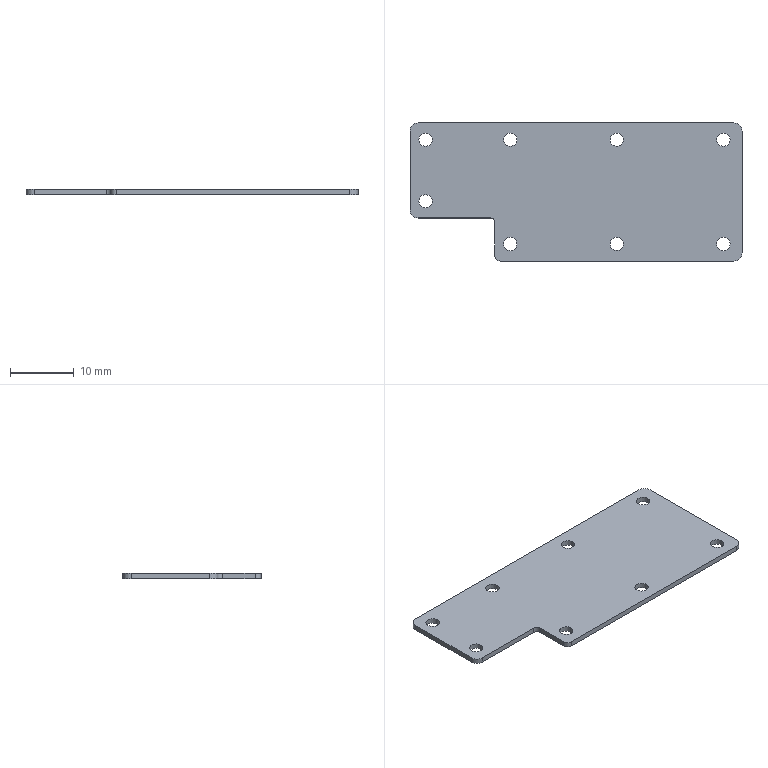Part | STEP file | Driver amplifier PA3PCB | 1 solid | 22 faces | box 52.1 x 21.66 x 0.832 mm | volume 840 mm3 | cylinder 14 | plane 8 | commonest cylinder face diameters 2.1 x8 2.54 x4 1.395 x1 1.8 x1